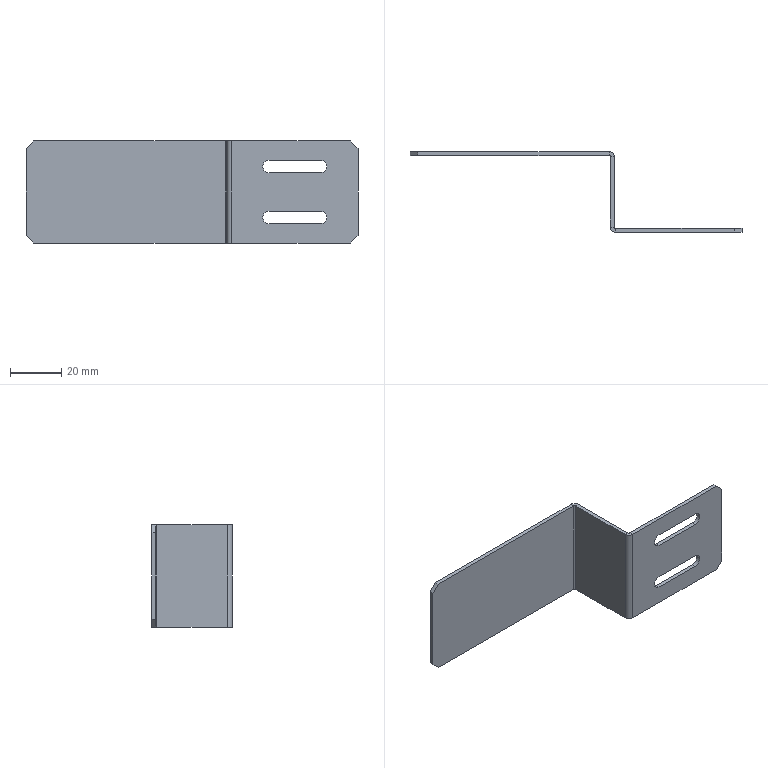Part | SolidWorks | features Chamfer 1, Cut 1, FlatPattern 1, SMBaseFlange 1, SheetMetal 1 | 1 solid | 34 faces | box 130 x 31.5 x 40 mm | volume 9150 mm3 | plane 26 | cylinder 8 | commonest cylinder face diameters 5 x4 1 x2 4 x2
STEP:
#1=CARTESIAN_POINT('',(0.,13.,20.));
#2=VERTEX_POINT('',#1);
#3=CARTESIAN_POINT('',(-1.5,13.,20.));
#4=VERTEX_POINT('',#3);
#5=CARTESIAN_POINT('',(0.,13.,20.));
#6=DIRECTION('',(-1.,0.,0.));
#7=VECTOR('',#6,1000.);
#8=LINE('',#5,#7);
#9=EDGE_CURVE('',#2,#4,#8,.T.);
#10=ORIENTED_EDGE('',*,*,#9,.F.);
#11=CARTESIAN_POINT('',(-2.,15.,20.));
#12=VERTEX_POINT('',#11);
#13=CARTESIAN_POINT('',(-2.,13.,20.));
#14=DIRECTION('',(0.,0.,-1.));
#15=DIRECTION('',(1.,0.,0.));
#16=AXIS2_PLACEMENT_3D('',#13,#14,#15);
#17=CIRCLE('',#16,2.);
#18=EDGE_CURVE('',#12,#2,#17,.T.);
#19=ORIENTED_EDGE('',*,*,#18,.F.);
#20=CARTESIAN_POINT('',(-2.,13.5,20.));
#21=VERTEX_POINT('',#20);
#22=CARTESIAN_POINT('',(-2.,13.5,20.));
#23=DIRECTION('',(0.,1.,0.));
#24=VECTOR('',#23,1000.);
#25=LINE('',#22,#24);
#26=EDGE_CURVE('',#21,#12,#25,.T.);
#27=ORIENTED_EDGE('',*,*,#26,.F.);
#28=CARTESIAN_POINT('',(-2.,13.,20.));
#29=DIRECTION('',(0.,0.,-1.));
#30=DIRECTION('',(1.,0.,0.));
#31=AXIS2_PLACEMENT_3D('',#28,#29,#30);
#32=CIRCLE('',#31,0.5);
#33=EDGE_CURVE('',#21,#4,#32,.T.);
#34=ORIENTED_EDGE('',*,*,#33,.T.);
#35=EDGE_LOOP('',(#10,#19,#27,#34));
#36=FACE_OUTER_BOUND('',#35,.T.);
#37=CARTESIAN_POINT('',(0.,13.,20.));
#38=DIRECTION('',(0.,0.,1.));
#39=DIRECTION('',(1.,0.,0.));
#40=AXIS2_PLACEMENT_3D('',#37,#38,#39);
#41=PLANE('',#40);
#42=ADVANCED_FACE('',(#36),#41,.T.);
#43=CARTESIAN_POINT('',(0.,-14.5,20.));
#44=VERTEX_POINT('',#43);
#45=CARTESIAN_POINT('',(0.,15.,20.));
#46=DIRECTION('',(0.,-1.,0.));
#47=VECTOR('',#46,1000.);
#48=LINE('',#45,#47);
#49=EDGE_CURVE('',#2,#44,#48,.T.);
#50=ORIENTED_EDGE('',*,*,#49,.F.);
#51=ORIENTED_EDGE('',*,*,#9,.T.);
#52=CARTESIAN_POINT('',(-1.5,-14.5,20.));
#53=VERTEX_POINT('',#52);
#54=CARTESIAN_POINT('',(-1.5,15.,20.));
#55=DIRECTION('',(0.,-1.,0.));
#56=VECTOR('',#55,1000.);
#57=LINE('',#54,#56);
#58=EDGE_CURVE('',#4,#53,#57,.T.);
#59=ORIENTED_EDGE('',*,*,#58,.T.);
#60=CARTESIAN_POINT('',(-1.5,-14.5,20.));
#61=DIRECTION('',(1.,0.,0.));
#62=VECTOR('',#61,1000.);
#63=LINE('',#60,#62);
#64=EDGE_CURVE('',#53,#44,#63,.T.);
#65=ORIENTED_EDGE('',*,*,#64,.T.);
#66=EDGE_LOOP('',(#50,#51,#59,#65));
#67=FACE_OUTER_BOUND('',#66,.T.);
#68=CARTESIAN_POINT('',(-2.,13.5,20.));
#69=DIRECTION('',(0.,0.,1.));
#70=DIRECTION('',(1.,0.,0.));
#71=AXIS2_PLACEMENT_3D('',#68,#69,#70);
#72=PLANE('',#71);
#73=ADVANCED_FACE('',(#67),#72,.T.);
#74=CARTESIAN_POINT('',(-2.,15.,-20.));
#75=VERTEX_POINT('',#74);
#76=CARTESIAN_POINT('',(-2.,13.5,-20.));
#77=VERTEX_POINT('',#76);
#78=CARTESIAN_POINT('',(-2.,15.,-20.));
#79=DIRECTION('',(0.,-1.,0.));
#80=VECTOR('',#79,1000.);
#81=LINE('',#78,#80);
#82=EDGE_CURVE('',#75,#77,#81,.T.);
#83=ORIENTED_EDGE('',*,*,#82,.F.);
#84=CARTESIAN_POINT('',(0.,13.,-20.));
#85=VERTEX_POINT('',#84);
#86=CARTESIAN_POINT('',(-2.,13.,-20.));
#87=DIRECTION('',(0.,0.,-1.));
#88=DIRECTION('',(1.,0.,0.));
#89=AXIS2_PLACEMENT_3D('',#86,#87,#88);
#90=CIRCLE('',#89,2.);
#91=EDGE_CURVE('',#75,#85,#90,.T.);
#92=ORIENTED_EDGE('',*,*,#91,.T.);
#93=CARTESIAN_POINT('',(-1.5,13.,-20.));
#94=VERTEX_POINT('',#93);
#95=CARTESIAN_POINT('',(-1.5,13.,-20.));
#96=DIRECTION('',(1.,0.,0.));
#97=VECTOR('',#96,1000.);
#98=LINE('',#95,#97);
#99=EDGE_CURVE('',#94,#85,#98,.T.);
#100=ORIENTED_EDGE('',*,*,#99,.F.);
#101=CARTESIAN_POINT('',(-2.,13.,-20.));
#102=DIRECTION('',(0.,0.,-1.));
#103=DIRECTION('',(1.,0.,0.));
#104=AXIS2_PLACEMENT_3D('',#101,#102,#103);
#105=CIRCLE('',#104,0.5);
#106=EDGE_CURVE('',#77,#94,#105,.T.);
#107=ORIENTED_EDGE('',*,*,#106,.F.);
#108=EDGE_LOOP('',(#83,#92,#100,#107));
#109=FACE_OUTER_BOUND('',#108,.T.);
#110=CARTESIAN_POINT('',(-2.,15.,-20.));
#111=DIRECTION('',(0.,0.,-1.));
#112=DIRECTION('',(-1.,0.,0.));
#113=AXIS2_PLACEMENT_3D('',#110,#111,#112);
#114=PLANE('',#113);
#115=ADVANCED_FACE('',(#109),#114,.T.);
#116=CARTESIAN_POINT('',(-77.,13.5,-20.));
#117=VERTEX_POINT('',#116);
#118=CARTESIAN_POINT('',(-80.,13.5,-20.));
#119=DIRECTION('',(1.,0.,0.));
#120=VECTOR('',#119,1000.);
#121=LINE('',#118,#120);
#122=EDGE_CURVE('',#117,#77,#121,.T.);
#123=ORIENTED_EDGE('',*,*,#122,.F.);
#124=CARTESIAN_POINT('',(-77.,15.,-20.));
#125=VERTEX_POINT('',#124);
#126=CARTESIAN_POINT('',(-77.,13.,-20.));
#127=DIRECTION('',(0.,1.,0.));
#128=VECTOR('',#127,1000.);
#129=LINE('',#126,#128);
#130=EDGE_CURVE('',#117,#125,#129,.T.);
#131=ORIENTED_EDGE('',*,*,#130,.T.);
#132=CARTESIAN_POINT('',(-80.,15.,-20.));
#133=DIRECTION('',(1.,0.,0.));
#134=VECTOR('',#133,1000.);
#135=LINE('',#132,#134);
#136=EDGE_CURVE('',#125,#75,#135,.T.);
#137=ORIENTED_EDGE('',*,*,#136,.T.);
#138=ORIENTED_EDGE('',*,*,#82,.T.);
#139=EDGE_LOOP('',(#123,#131,#137,#138));
#140=FACE_OUTER_BOUND('',#139,.T.);
#141=CARTESIAN_POINT('',(-1.5,13.,-20.));
#142=DIRECTION('',(0.,0.,-1.));
#143=DIRECTION('',(-1.,0.,0.));
#144=AXIS2_PLACEMENT_3D('',#141,#142,#143);
#145=PLANE('',#144);
#146=ADVANCED_FACE('',(#140),#145,.T.);
#147=CARTESIAN_POINT('',(0.5,-15.,20.));
#148=VERTEX_POINT('',#147);
#149=CARTESIAN_POINT('',(0.5,-16.5,20.));
#150=VERTEX_POINT('',#149);
#151=CARTESIAN_POINT('',(0.5,-15.,20.));
#152=DIRECTION('',(0.,-1.,0.));
#153=VECTOR('',#152,1000.);
#154=LINE('',#151,#153);
#155=EDGE_CURVE('',#148,#150,#154,.T.);
#156=ORIENTED_EDGE('',*,*,#155,.F.);
#157=CARTESIAN_POINT('',(0.5,-14.5,20.));
#158=DIRECTION('',(0.,0.,1.));
#159=DIRECTION('',(-1.,0.,0.));
#160=AXIS2_PLACEMENT_3D('',#157,#158,#159);
#161=CIRCLE('',#160,0.5);
#162=EDGE_CURVE('',#44,#148,#161,.T.);
#163=ORIENTED_EDGE('',*,*,#162,.F.);
#164=ORIENTED_EDGE('',*,*,#64,.F.);
#165=CARTESIAN_POINT('',(0.5,-14.5,20.));
#166=DIRECTION('',(0.,0.,1.));
#167=DIRECTION('',(1.,0.,0.));
#168=AXIS2_PLACEMENT_3D('',#165,#166,#167);
#169=CIRCLE('',#168,2.);
#170=EDGE_CURVE('',#53,#150,#169,.T.);
#171=ORIENTED_EDGE('',*,*,#170,.T.);
#172=EDGE_LOOP('',(#156,#163,#164,#171));
#173=FACE_OUTER_BOUND('',#172,.T.);
#174=CARTESIAN_POINT('',(0.5,-15.,20.));
#175=DIRECTION('',(0.,0.,1.));
#176=DIRECTION('',(1.,0.,0.));
#177=AXIS2_PLACEMENT_3D('',#174,#175,#176);
#178=PLANE('',#177);
#179=ADVANCED_FACE('',(#173),#178,.T.);
#180=CARTESIAN_POINT('',(47.,-16.5,20.));
#181=VERTEX_POINT('',#180);
#182=CARTESIAN_POINT('',(0.,-16.5,20.));
#183=DIRECTION('',(1.,0.,0.));
#184=VECTOR('',#183,1000.);
#185=LINE('',#182,#184);
#186=EDGE_CURVE('',#150,#181,#185,.T.);
#187=ORIENTED_EDGE('',*,*,#186,.T.);
#188=CARTESIAN_POINT('',(47.,-15.,20.));
#189=VERTEX_POINT('',#188);
#190=CARTESIAN_POINT('',(47.,-14.5,20.));
#191=DIRECTION('',(0.,1.,0.));
#192=VECTOR('',#191,1000.);
#193=LINE('',#190,#192);
#194=EDGE_CURVE('',#181,#189,#193,.T.);
#195=ORIENTED_EDGE('',*,*,#194,.T.);
#196=CARTESIAN_POINT('',(0.,-15.,20.));
#197=DIRECTION('',(1.,0.,0.));
#198=VECTOR('',#197,1000.);
#199=LINE('',#196,#198);
#200=EDGE_CURVE('',#148,#189,#199,.T.);
#201=ORIENTED_EDGE('',*,*,#200,.F.);
#202=ORIENTED_EDGE('',*,*,#155,.T.);
#203=EDGE_LOOP('',(#187,#195,#201,#202));
#204=FACE_OUTER_BOUND('',#203,.T.);
#205=CARTESIAN_POINT('',(-1.5,-14.5,20.));
#206=DIRECTION('',(0.,0.,1.));
#207=DIRECTION('',(1.,0.,0.));
#208=AXIS2_PLACEMENT_3D('',#205,#206,#207);
#209=PLANE('',#208);
#210=ADVANCED_FACE('',(#204),#209,.T.);
#211=CARTESIAN_POINT('',(0.,-14.5,-20.));
#212=VERTEX_POINT('',#211);
#213=CARTESIAN_POINT('',(-1.5,-14.5,-20.));
#214=VERTEX_POINT('',#213);
#215=CARTESIAN_POINT('',(0.,-14.5,-20.));
#216=DIRECTION('',(-1.,0.,0.));
#217=VECTOR('',#216,1000.);
#218=LINE('',#215,#217);
#219=EDGE_CURVE('',#212,#214,#218,.T.);
#220=ORIENTED_EDGE('',*,*,#219,.F.);
#221=CARTESIAN_POINT('',(0.5,-15.,-20.));
#222=VERTEX_POINT('',#221);
#223=CARTESIAN_POINT('',(0.5,-14.5,-20.));
#224=DIRECTION('',(0.,0.,1.));
#225=DIRECTION('',(-1.,0.,0.));
#226=AXIS2_PLACEMENT_3D('',#223,#224,#225);
#227=CIRCLE('',#226,0.5);
#228=EDGE_CURVE('',#212,#222,#227,.T.);
#229=ORIENTED_EDGE('',*,*,#228,.T.);
#230=CARTESIAN_POINT('',(0.5,-16.5,-20.));
#231=VERTEX_POINT('',#230);
#232=CARTESIAN_POINT('',(0.5,-16.5,-20.));
#233=DIRECTION('',(0.,1.,0.));
#234=VECTOR('',#233,1000.);
#235=LINE('',#232,#234);
#236=EDGE_CURVE('',#231,#222,#235,.T.);
#237=ORIENTED_EDGE('',*,*,#236,.F.);
#238=CARTESIAN_POINT('',(0.5,-14.5,-20.));
#239=DIRECTION('',(0.,0.,1.));
#240=DIRECTION('',(1.,0.,0.));
#241=AXIS2_PLACEMENT_3D('',#238,#239,#240);
#242=CIRCLE('',#241,2.);
#243=EDGE_CURVE('',#214,#231,#242,.T.);
#244=ORIENTED_EDGE('',*,*,#243,.F.);
#245=EDGE_LOOP('',(#220,#229,#237,#244));
#246=FACE_OUTER_BOUND('',#245,.T.);
#247=CARTESIAN_POINT('',(0.,-14.5,-20.));
#248=DIRECTION('',(0.,0.,-1.));
#249=DIRECTION('',(-1.,0.,0.));
#250=AXIS2_PLACEMENT_3D('',#247,#248,#249);
#251=PLANE('',#250);
#252=ADVANCED_FACE('',(#246),#251,.T.);
#253=CARTESIAN_POINT('',(0.,15.,-20.));
#254=DIRECTION('',(0.,-1.,0.));
#255=VECTOR('',#254,1000.);
#256=LINE('',#253,#255);
#257=EDGE_CURVE('',#85,#212,#256,.T.);
#258=ORIENTED_EDGE('',*,*,#257,.T.);
#259=ORIENTED_EDGE('',*,*,#219,.T.);
#260=CARTESIAN_POINT('',(-1.5,15.,-20.));
#261=DIRECTION('',(0.,-1.,0.));
#262=VECTOR('',#261,1000.);
#263=LINE('',#260,#262);
#264=EDGE_CURVE('',#94,#214,#263,.T.);
#265=ORIENTED_EDGE('',*,*,#264,.F.);
#266=ORIENTED_EDGE('',*,*,#99,.T.);
#267=EDGE_LOOP('',(#258,#259,#265,#266));
#268=FACE_OUTER_BOUND('',#267,.T.);
#269=CARTESIAN_POINT('',(0.5,-16.5,-20.));
#270=DIRECTION('',(0.,0.,-1.));
#271=DIRECTION('',(-1.,0.,0.));
#272=AXIS2_PLACEMENT_3D('',#269,#270,#271);
#273=PLANE('',#272);
#274=ADVANCED_FACE('',(#268),#273,.T.);
#275=CARTESIAN_POINT('',(15.25,-16.5,12.5));
#276=VERTEX_POINT('',#275);
#277=CARTESIAN_POINT('',(35.25,-16.5,12.5));
#278=VERTEX_POINT('',#277);
#279=CARTESIAN_POINT('',(35.25,-16.5,12.5));
#280=DIRECTION('',(1.,0.,0.));
#281=VECTOR('',#280,1000.);
#282=LINE('',#279,#281);
#283=EDGE_CURVE('',#276,#278,#282,.T.);
#284=ORIENTED_EDGE('',*,*,#283,.T.);
#285=CARTESIAN_POINT('',(35.25,-16.5,7.5));
#286=VERTEX_POINT('',#285);
#287=CARTESIAN_POINT('',(35.25,-16.5,10.));
#288=DIRECTION('',(0.,1.,0.));
#289=DIRECTION('',(0.,0.,1.));
#290=AXIS2_PLACEMENT_3D('',#287,#288,#289);
#291=CIRCLE('',#290,2.5);
#292=EDGE_CURVE('',#278,#286,#291,.T.);
#293=ORIENTED_EDGE('',*,*,#292,.T.);
#294=CARTESIAN_POINT('',(15.25,-16.5,7.5));
#295=VERTEX_POINT('',#294);
#296=CARTESIAN_POINT('',(35.25,-16.5,7.5));
#297=DIRECTION('',(-1.,0.,0.));
#298=VECTOR('',#297,1000.);
#299=LINE('',#296,#298);
#300=EDGE_CURVE('',#286,#295,#299,.T.);
#301=ORIENTED_EDGE('',*,*,#300,.T.);
#302=CARTESIAN_POINT('',(15.25,-16.5,10.));
#303=DIRECTION('',(0.,1.,0.));
#304=DIRECTION('',(0.,0.,1.));
#305=AXIS2_PLACEMENT_3D('',#302,#303,#304);
#306=CIRCLE('',#305,2.5);
#307=EDGE_CURVE('',#295,#276,#306,.T.);
#308=ORIENTED_EDGE('',*,*,#307,.T.);
#309=EDGE_LOOP('',(#284,#293,#301,#308));
#310=FACE_BOUND('',#309,.T.);
#311=CARTESIAN_POINT('',(15.25,-16.5,-7.5));
#312=VERTEX_POINT('',#311);
#313=CARTESIAN_POINT('',(35.25,-16.5,-7.5));
#314=VERTEX_POINT('',#313);
#315=CARTESIAN_POINT('',(35.25,-16.5,-7.5));
#316=DIRECTION('',(1.,0.,0.));
#317=VECTOR('',#316,1000.);
#318=LINE('',#315,#317);
#319=EDGE_CURVE('',#312,#314,#318,.T.);
#320=ORIENTED_EDGE('',*,*,#319,.T.);
#321=CARTESIAN_POINT('',(35.25,-16.5,-12.5));
#322=VERTEX_POINT('',#321);
#323=CARTESIAN_POINT('',(35.25,-16.5,-10.));
#324=DIRECTION('',(0.,1.,0.));
#325=DIRECTION('',(0.,0.,1.));
#326=AXIS2_PLACEMENT_3D('',#323,#324,#325);
#327=CIRCLE('',#326,2.5);
#328=EDGE_CURVE('',#314,#322,#327,.T.);
#329=ORIENTED_EDGE('',*,*,#328,.T.);
#330=CARTESIAN_POINT('',(15.25,-16.5,-12.5));
#331=VERTEX_POINT('',#330);
#332=CARTESIAN_POINT('',(35.25,-16.5,-12.5));
#333=DIRECTION('',(-1.,0.,0.));
#334=VECTOR('',#333,1000.);
#335=LINE('',#332,#334);
#336=EDGE_CURVE('',#322,#331,#335,.T.);
#337=ORIENTED_EDGE('',*,*,#336,.T.);
#338=CARTESIAN_POINT('',(15.25,-16.5,-10.));
#339=DIRECTION('',(0.,1.,0.));
#340=DIRECTION('',(0.,0.,1.));
#341=AXIS2_PLACEMENT_3D('',#338,#339,#340);
#342=CIRCLE('',#341,2.5);
#343=EDGE_CURVE('',#331,#312,#342,.T.);
#344=ORIENTED_EDGE('',*,*,#343,.T.);
#345=EDGE_LOOP('',(#320,#329,#337,#344));
#346=FACE_BOUND('',#345,.T.);
#347=CARTESIAN_POINT('',(47.,-16.5,-20.));
#348=VERTEX_POINT('',#347);
#349=CARTESIAN_POINT('',(0.,-16.5,-20.));
#350=DIRECTION('',(1.,0.,0.));
#351=VECTOR('',#350,1000.);
#352=LINE('',#349,#351);
#353=EDGE_CURVE('',#231,#348,#352,.T.);
#354=ORIENTED_EDGE('',*,*,#353,.T.);
#355=CARTESIAN_POINT('',(50.,-16.5,-17.));
#356=VERTEX_POINT('',#355);
#357=CARTESIAN_POINT('',(47.,-16.5,-20.));
#358=DIRECTION('',(0.7071,0.,0.7071));
#359=VECTOR('',#358,1000.);
#360=LINE('',#357,#359);
#361=EDGE_CURVE('',#348,#356,#360,.T.);
#362=ORIENTED_EDGE('',*,*,#361,.T.);
#363=CARTESIAN_POINT('',(50.,-16.5,17.));
#364=VERTEX_POINT('',#363);
#365=CARTESIAN_POINT('',(50.,-16.5,20.));
#366=DIRECTION('',(0.,0.,-1.));
#367=VECTOR('',#366,1000.);
#368=LINE('',#365,#367);
#369=EDGE_CURVE('',#364,#356,#368,.T.);
#370=ORIENTED_EDGE('',*,*,#369,.F.);
#371=CARTESIAN_POINT('',(50.,-16.5,17.));
#372=DIRECTION('',(-0.7071,0.,0.7071));
#373=VECTOR('',#372,1000.);
#374=LINE('',#371,#373);
#375=EDGE_CURVE('',#364,#181,#374,.T.);
#376=ORIENTED_EDGE('',*,*,#375,.T.);
#377=ORIENTED_EDGE('',*,*,#186,.F.);
#378=CARTESIAN_POINT('',(0.5,-16.5,20.));
#379=DIRECTION('',(0.,0.,-1.));
#380=VECTOR('',#379,1000.);
#381=LINE('',#378,#380);
#382=EDGE_CURVE('',#150,#231,#381,.T.);
#383=ORIENTED_EDGE('',*,*,#382,.T.);
#384=EDGE_LOOP('',(#354,#362,#370,#376,#377,#383));
#385=FACE_OUTER_BOUND('',#384,.T.);
#386=CARTESIAN_POINT('',(0.,-16.5,20.));
#387=DIRECTION('',(0.,1.,0.));
#388=DIRECTION('',(0.,0.,1.));
#389=AXIS2_PLACEMENT_3D('',#386,#387,#388);
#390=PLANE('',#389);
#391=ADVANCED_FACE('',(#310,#346,#385),#390,.F.);
#392=ORIENTED_EDGE('',*,*,#369,.T.);
#393=CARTESIAN_POINT('',(50.,-15.,-17.));
#394=VERTEX_POINT('',#393);
#395=CARTESIAN_POINT('',(50.,-15.,-17.));
#396=DIRECTION('',(0.,1.,0.));
#397=VECTOR('',#396,1000.);
#398=LINE('',#395,#397);
#399=EDGE_CURVE('',#356,#394,#398,.T.);
#400=ORIENTED_EDGE('',*,*,#399,.T.);
#401=CARTESIAN_POINT('',(50.,-15.,17.));
#402=VERTEX_POINT('',#401);
#403=CARTESIAN_POINT('',(50.,-15.,20.));
#404=DIRECTION('',(0.,0.,-1.));
#405=VECTOR('',#404,1000.);
#406=LINE('',#403,#405);
#407=EDGE_CURVE('',#402,#394,#406,.T.);
#408=ORIENTED_EDGE('',*,*,#407,.F.);
#409=CARTESIAN_POINT('',(50.,-15.,17.));
#410=DIRECTION('',(0.,-1.,0.));
#411=VECTOR('',#410,1000.);
#412=LINE('',#409,#411);
#413=EDGE_CURVE('',#402,#364,#412,.T.);
#414=ORIENTED_EDGE('',*,*,#413,.T.);
#415=EDGE_LOOP('',(#392,#400,#408,#414));
#416=FACE_OUTER_BOUND('',#415,.T.);
#417=CARTESIAN_POINT('',(50.,-15.,20.));
#418=DIRECTION('',(1.,0.,0.));
#419=DIRECTION('',(0.,0.,-1.));
#420=AXIS2_PLACEMENT_3D('',#417,#418,#419);
#421=PLANE('',#420);
#422=ADVANCED_FACE('',(#416),#421,.T.);
#423=CARTESIAN_POINT('',(35.25,-15.,12.5));
#424=VERTEX_POINT('',#423);
#425=CARTESIAN_POINT('',(35.25,-15.,7.5));
#426=VERTEX_POINT('',#425);
#427=CARTESIAN_POINT('',(35.25,-15.,10.));
#428=DIRECTION('',(0.,1.,0.));
#429=DIRECTION('',(0.,0.,1.));
#430=AXIS2_PLACEMENT_3D('',#427,#428,#429);
#431=CIRCLE('',#430,2.5);
#432=EDGE_CURVE('',#424,#426,#431,.T.);
#433=ORIENTED_EDGE('',*,*,#432,.F.);
#434=CARTESIAN_POINT('',(15.25,-15.,12.5));
#435=VERTEX_POINT('',#434);
#436=CARTESIAN_POINT('',(35.25,-15.,12.5));
#437=DIRECTION('',(1.,0.,0.));
#438=VECTOR('',#437,1000.);
#439=LINE('',#436,#438);
#440=EDGE_CURVE('',#435,#424,#439,.T.);
#441=ORIENTED_EDGE('',*,*,#440,.F.);
#442=CARTESIAN_POINT('',(15.25,-15.,7.5));
#443=VERTEX_POINT('',#442);
#444=CARTESIAN_POINT('',(15.25,-15.,10.));
#445=DIRECTION('',(0.,1.,0.));
#446=DIRECTION('',(0.,0.,1.));
#447=AXIS2_PLACEMENT_3D('',#444,#445,#446);
#448=CIRCLE('',#447,2.5);
#449=EDGE_CURVE('',#443,#435,#448,.T.);
#450=ORIENTED_EDGE('',*,*,#449,.F.);
#451=CARTESIAN_POINT('',(35.25,-15.,7.5));
#452=DIRECTION('',(-1.,0.,0.));
#453=VECTOR('',#452,1000.);
#454=LINE('',#451,#453);
#455=EDGE_CURVE('',#426,#443,#454,.T.);
#456=ORIENTED_EDGE('',*,*,#455,.F.);
#457=EDGE_LOOP('',(#433,#441,#450,#456));
#458=FACE_BOUND('',#457,.T.);
#459=CARTESIAN_POINT('',(35.25,-15.,-7.5));
#460=VERTEX_POINT('',#459);
#461=CARTESIAN_POINT('',(35.25,-15.,-12.5));
#462=VERTEX_POINT('',#461);
#463=CARTESIAN_POINT('',(35.25,-15.,-10.));
#464=DIRECTION('',(0.,1.,0.));
#465=DIRECTION('',(0.,0.,1.));
#466=AXIS2_PLACEMENT_3D('',#463,#464,#465);
#467=CIRCLE('',#466,2.5);
#468=EDGE_CURVE('',#460,#462,#467,.T.);
#469=ORIENTED_EDGE('',*,*,#468,.F.);
#470=CARTESIAN_POINT('',(15.25,-15.,-7.5));
#471=VERTEX_POINT('',#470);
#472=CARTESIAN_POINT('',(35.25,-15.,-7.5));
#473=DIRECTION('',(1.,0.,0.));
#474=VECTOR('',#473,1000.);
#475=LINE('',#472,#474);
#476=EDGE_CURVE('',#471,#460,#475,.T.);
#477=ORIENTED_EDGE('',*,*,#476,.F.);
#478=CARTESIAN_POINT('',(15.25,-15.,-12.5));
#479=VERTEX_POINT('',#478);
#480=CARTESIAN_POINT('',(15.25,-15.,-10.));
#481=DIRECTION('',(0.,1.,0.));
#482=DIRECTION('',(0.,0.,1.));
#483=AXIS2_PLACEMENT_3D('',#480,#481,#482);
#484=CIRCLE('',#483,2.5);
#485=EDGE_CURVE('',#479,#471,#484,.T.);
#486=ORIENTED_EDGE('',*,*,#485,.F.);
#487=CARTESIAN_POINT('',(35.25,-15.,-12.5));
#488=DIRECTION('',(-1.,0.,0.));
#489=VECTOR('',#488,1000.);
#490=LINE('',#487,#489);
#491=EDGE_CURVE('',#462,#479,#490,.T.);
#492=ORIENTED_EDGE('',*,*,#491,.F.);
#493=EDGE_LOOP('',(#469,#477,#486,#492));
#494=FACE_BOUND('',#493,.T.);
#495=ORIENTED_EDGE('',*,*,#407,.T.);
#496=CARTESIAN_POINT('',(47.,-15.,-20.));
#497=VERTEX_POINT('',#496);
#498=CARTESIAN_POINT('',(43.5,-15.,-23.5));
#499=DIRECTION('',(-0.7071,0.,-0.7071));
#500=VECTOR('',#499,1000.);
#501=LINE('',#498,#500);
#502=EDGE_CURVE('',#394,#497,#501,.T.);
#503=ORIENTED_EDGE('',*,*,#502,.T.);
#504=CARTESIAN_POINT('',(0.,-15.,-20.));
#505=DIRECTION('',(1.,0.,0.));
#506=VECTOR('',#505,1000.);
#507=LINE('',#504,#506);
#508=EDGE_CURVE('',#222,#497,#507,.T.);
#509=ORIENTED_EDGE('',*,*,#508,.F.);
#510=CARTESIAN_POINT('',(0.5,-15.,20.));
#511=DIRECTION('',(0.,0.,-1.));
#512=VECTOR('',#511,1000.);
#513=LINE('',#510,#512);
#514=EDGE_CURVE('',#148,#222,#513,.T.);
#515=ORIENTED_EDGE('',*,*,#514,.F.);
#516=ORIENTED_EDGE('',*,*,#200,.T.);
#517=CARTESIAN_POINT('',(23.5,-15.,43.5));
#518=DIRECTION('',(0.7071,0.,-0.7071));
#519=VECTOR('',#518,1000.);
#520=LINE('',#517,#519);
#521=EDGE_CURVE('',#189,#402,#520,.T.);
#522=ORIENTED_EDGE('',*,*,#521,.T.);
#523=EDGE_LOOP('',(#495,#503,#509,#515,#516,#522));
#524=FACE_OUTER_BOUND('',#523,.T.);
#525=CARTESIAN_POINT('',(0.,-15.,20.));
#526=DIRECTION('',(0.,1.,0.));
#527=DIRECTION('',(0.,0.,1.));
#528=AXIS2_PLACEMENT_3D('',#525,#526,#527);
#529=PLANE('',#528);
#530=ADVANCED_FACE('',(#458,#494,#524),#529,.T.);
#531=ORIENTED_EDGE('',*,*,#228,.F.);
#532=CARTESIAN_POINT('',(0.,-14.5,20.));
#533=DIRECTION('',(0.,0.,-1.));
#534=VECTOR('',#533,1000.);
#535=LINE('',#532,#534);
#536=EDGE_CURVE('',#44,#212,#535,.T.);
#537=ORIENTED_EDGE('',*,*,#536,.F.);
#538=ORIENTED_EDGE('',*,*,#162,.T.);
#539=ORIENTED_EDGE('',*,*,#514,.T.);
#540=EDGE_LOOP('',(#531,#537,#538,#539));
#541=FACE_OUTER_BOUND('',#540,.T.);
#542=CARTESIAN_POINT('',(0.5,-14.5,20.));
#543=DIRECTION('',(0.,0.,-1.));
#544=DIRECTION('',(-1.,0.,0.));
#545=AXIS2_PLACEMENT_3D('',#542,#543,#544);
#546=CYLINDRICAL_SURFACE('',#545,0.5);
#547=ADVANCED_FACE('',(#541),#546,.F.);
#548=ORIENTED_EDGE('',*,*,#257,.F.);
#549=CARTESIAN_POINT('',(0.,13.,20.));
#550=DIRECTION('',(0.,0.,-1.));
#551=VECTOR('',#550,1000.);
#552=LINE('',#549,#551);
#553=EDGE_CURVE('',#2,#85,#552,.T.);
#554=ORIENTED_EDGE('',*,*,#553,.F.);
#555=ORIENTED_EDGE('',*,*,#49,.T.);
#556=ORIENTED_EDGE('',*,*,#536,.T.);
#557=EDGE_LOOP('',(#548,#554,#555,#556));
#558=FACE_OUTER_BOUND('',#557,.T.);
#559=CARTESIAN_POINT('',(0.,15.,20.));
#560=DIRECTION('',(1.,0.,0.));
#561=DIRECTION('',(0.,0.,-1.));
#562=AXIS2_PLACEMENT_3D('',#559,#560,#561);
#563=PLANE('',#562);
#564=ADVANCED_FACE('',(#558),#563,.T.);
#565=ORIENTED_EDGE('',*,*,#91,.F.);
#566=CARTESIAN_POINT('',(-2.,15.,20.));
#567=DIRECTION('',(0.,0.,-1.));
#568=VECTOR('',#567,1000.);
#569=LINE('',#566,#568);
#570=EDGE_CURVE('',#12,#75,#569,.T.);
#571=ORIENTED_EDGE('',*,*,#570,.F.);
#572=ORIENTED_EDGE('',*,*,#18,.T.);
#573=ORIENTED_EDGE('',*,*,#553,.T.);
#574=EDGE_LOOP('',(#565,#571,#572,#573));
#575=FACE_OUTER_BOUND('',#574,.T.);
#576=CARTESIAN_POINT('',(-2.,13.,20.));
#577=DIRECTION('',(0.,0.,-1.));
#578=DIRECTION('',(-1.,0.,0.));
#579=AXIS2_PLACEMENT_3D('',#576,#577,#578);
#580=CYLINDRICAL_SURFACE('',#579,2.);
#581=ADVANCED_FACE('',(#575),#580,.T.);
#582=ORIENTED_EDGE('',*,*,#136,.F.);
#583=CARTESIAN_POINT('',(-80.,15.,-17.));
#584=VERTEX_POINT('',#583);
#585=CARTESIAN_POINT('',(-98.5,15.,1.5));
#586=DIRECTION('',(-0.7071,0.,0.7071));
#587=VECTOR('',#586,1000.);
#588=LINE('',#585,#587);
#589=EDGE_CURVE('',#125,#584,#588,.T.);
#590=ORIENTED_EDGE('',*,*,#589,.T.);
#591=CARTESIAN_POINT('',(-80.,15.,17.));
#592=VERTEX_POINT('',#591);
#593=CARTESIAN_POINT('',(-80.,15.,20.));
#594=DIRECTION('',(0.,0.,-1.));
#595=VECTOR('',#594,1000.);
#596=LINE('',#593,#595);
#597=EDGE_CURVE('',#592,#584,#596,.T.);
#598=ORIENTED_EDGE('',*,*,#597,.F.);
#599=CARTESIAN_POINT('',(-77.,15.,20.));
#600=VERTEX_POINT('',#599);
#601=CARTESIAN_POINT('',(-78.5,15.,18.5));
#602=DIRECTION('',(0.7071,0.,0.7071));
#603=VECTOR('',#602,1000.);
#604=LINE('',#601,#603);
#605=EDGE_CURVE('',#592,#600,#604,.T.);
#606=ORIENTED_EDGE('',*,*,#605,.T.);
#607=CARTESIAN_POINT('',(-80.,15.,20.));
#608=DIRECTION('',(1.,0.,0.));
#609=VECTOR('',#608,1000.);
#610=LINE('',#607,#609);
#611=EDGE_CURVE('',#600,#12,#610,.T.);
#612=ORIENTED_EDGE('',*,*,#611,.T.);
#613=ORIENTED_EDGE('',*,*,#570,.T.);
#614=EDGE_LOOP('',(#582,#590,#598,#606,#612,#613));
#615=FACE_OUTER_BOUND('',#614,.T.);
#616=CARTESIAN_POINT('',(-80.,15.,20.));
#617=DIRECTION('',(0.,1.,0.));
#618=DIRECTION('',(0.,0.,1.));
#619=AXIS2_PLACEMENT_3D('',#616,#617,#618);
#620=PLANE('',#619);
#621=ADVANCED_FACE('',(#615),#620,.T.);
#622=ORIENTED_EDGE('',*,*,#597,.T.);
#623=CARTESIAN_POINT('',(-80.,13.5,-17.));
#624=VERTEX_POINT('',#623);
#625=CARTESIAN_POINT('',(-80.,13.5,-17.));
#626=DIRECTION('',(0.,-1.,0.));
#627=VECTOR('',#626,1000.);
#628=LINE('',#625,#627);
#629=EDGE_CURVE('',#584,#624,#628,.T.);
#630=ORIENTED_EDGE('',*,*,#629,.T.);
#631=CARTESIAN_POINT('',(-80.,13.5,17.));
#632=VERTEX_POINT('',#631);
#633=CARTESIAN_POINT('',(-80.,13.5,20.));
#634=DIRECTION('',(0.,0.,-1.));
#635=VECTOR('',#634,1000.);
#636=LINE('',#633,#635);
#637=EDGE_CURVE('',#632,#624,#636,.T.);
#638=ORIENTED_EDGE('',*,*,#637,.F.);
#639=CARTESIAN_POINT('',(-80.,15.,17.));
#640=DIRECTION('',(0.,1.,0.));
#641=VECTOR('',#640,1000.);
#642=LINE('',#639,#641);
#643=EDGE_CURVE('',#632,#592,#642,.T.);
#644=ORIENTED_EDGE('',*,*,#643,.T.);
#645=EDGE_LOOP('',(#622,#630,#638,#644));
#646=FACE_OUTER_BOUND('',#645,.T.);
#647=CARTESIAN_POINT('',(-80.,13.5,20.));
#648=DIRECTION('',(-1.,0.,0.));
#649=DIRECTION('',(0.,0.,1.));
#650=AXIS2_PLACEMENT_3D('',#647,#648,#649);
#651=PLANE('',#650);
#652=ADVANCED_FACE('',(#646),#651,.T.);
#653=ORIENTED_EDGE('',*,*,#637,.T.);
#654=CARTESIAN_POINT('',(-77.,13.5,-20.));
#655=DIRECTION('',(0.7071,0.,-0.7071));
#656=VECTOR('',#655,1000.);
#657=LINE('',#654,#656);
#658=EDGE_CURVE('',#624,#117,#657,.T.);
#659=ORIENTED_EDGE('',*,*,#658,.T.);
#660=ORIENTED_EDGE('',*,*,#122,.T.);
#661=CARTESIAN_POINT('',(-2.,13.5,20.));
#662=DIRECTION('',(0.,0.,-1.));
#663=VECTOR('',#662,1000.);
#664=LINE('',#661,#663);
#665=EDGE_CURVE('',#21,#77,#664,.T.);
#666=ORIENTED_EDGE('',*,*,#665,.F.);
#667=CARTESIAN_POINT('',(-77.,13.5,20.));
#668=VERTEX_POINT('',#667);
#669=CARTESIAN_POINT('',(-80.,13.5,20.));
#670=DIRECTION('',(1.,0.,0.));
#671=VECTOR('',#670,1000.);
#672=LINE('',#669,#671);
#673=EDGE_CURVE('',#668,#21,#672,.T.);
#674=ORIENTED_EDGE('',*,*,#673,.F.);
#675=CARTESIAN_POINT('',(-80.,13.5,17.));
#676=DIRECTION('',(-0.7071,0.,-0.7071));
#677=VECTOR('',#676,1000.);
#678=LINE('',#675,#677);
#679=EDGE_CURVE('',#668,#632,#678,.T.);
#680=ORIENTED_EDGE('',*,*,#679,.T.);
#681=EDGE_LOOP('',(#653,#659,#660,#666,#674,#680));
#682=FACE_OUTER_BOUND('',#681,.T.);
#683=CARTESIAN_POINT('',(-80.,13.5,20.));
#684=DIRECTION('',(0.,1.,0.));
#685=DIRECTION('',(0.,0.,1.));
#686=AXIS2_PLACEMENT_3D('',#683,#684,#685);
#687=PLANE('',#686);
#688=ADVANCED_FACE('',(#682),#687,.F.);
#689=ORIENTED_EDGE('',*,*,#106,.T.);
#690=CARTESIAN_POINT('',(-1.5,13.,20.));
#691=DIRECTION('',(0.,0.,-1.));
#692=VECTOR('',#691,1000.);
#693=LINE('',#690,#692);
#694=EDGE_CURVE('',#4,#94,#693,.T.);
#695=ORIENTED_EDGE('',*,*,#694,.F.);
#696=ORIENTED_EDGE('',*,*,#33,.F.);
#697=ORIENTED_EDGE('',*,*,#665,.T.);
#698=EDGE_LOOP('',(#689,#695,#696,#697));
#699=FACE_OUTER_BOUND('',#698,.T.);
#700=CARTESIAN_POINT('',(-2.,13.,20.));
#701=DIRECTION('',(0.,0.,-1.));
#702=DIRECTION('',(-1.,0.,0.));
#703=AXIS2_PLACEMENT_3D('',#700,#701,#702);
#704=CYLINDRICAL_SURFACE('',#703,0.5);
#705=ADVANCED_FACE('',(#699),#704,.F.);
#706=ORIENTED_EDGE('',*,*,#264,.T.);
#707=CARTESIAN_POINT('',(-1.5,-14.5,20.));
#708=DIRECTION('',(0.,0.,-1.));
#709=VECTOR('',#708,1000.);
#710=LINE('',#707,#709);
#711=EDGE_CURVE('',#53,#214,#710,.T.);
#712=ORIENTED_EDGE('',*,*,#711,.F.);
#713=ORIENTED_EDGE('',*,*,#58,.F.);
#714=ORIENTED_EDGE('',*,*,#694,.T.);
#715=EDGE_LOOP('',(#706,#712,#713,#714));
#716=FACE_OUTER_BOUND('',#715,.T.);
#717=CARTESIAN_POINT('',(-1.5,15.,20.));
#718=DIRECTION('',(1.,0.,0.));
#719=DIRECTION('',(0.,0.,-1.));
#720=AXIS2_PLACEMENT_3D('',#717,#718,#719);
#721=PLANE('',#720);
#722=ADVANCED_FACE('',(#716),#721,.F.);
#723=ORIENTED_EDGE('',*,*,#243,.T.);
#724=ORIENTED_EDGE('',*,*,#382,.F.);
#725=ORIENTED_EDGE('',*,*,#170,.F.);
#726=ORIENTED_EDGE('',*,*,#711,.T.);
#727=EDGE_LOOP('',(#723,#724,#725,#726));
#728=FACE_OUTER_BOUND('',#727,.T.);
#729=CARTESIAN_POINT('',(0.5,-14.5,20.));
#730=DIRECTION('',(0.,0.,-1.));
#731=DIRECTION('',(-1.,0.,0.));
#732=AXIS2_PLACEMENT_3D('',#729,#730,#731);
#733=CYLINDRICAL_SURFACE('',#732,2.);
#734=ADVANCED_FACE('',(#728),#733,.T.);
#735=ORIENTED_EDGE('',*,*,#611,.F.);
#736=CARTESIAN_POINT('',(-77.,13.5,20.));
#737=DIRECTION('',(0.,-1.,0.));
#738=VECTOR('',#737,1000.);
#739=LINE('',#736,#738);
#740=EDGE_CURVE('',#600,#668,#739,.T.);
#741=ORIENTED_EDGE('',*,*,#740,.T.);
#742=ORIENTED_EDGE('',*,*,#673,.T.);
#743=ORIENTED_EDGE('',*,*,#26,.T.);
#744=EDGE_LOOP('',(#735,#741,#742,#743));
#745=FACE_OUTER_BOUND('',#744,.T.);
#746=CARTESIAN_POINT('',(0.5,-14.5,20.));
#747=DIRECTION('',(0.,0.,-1.));
#748=DIRECTION('',(-1.,0.,0.));
#749=AXIS2_PLACEMENT_3D('',#746,#747,#748);
#750=PLANE('',#749);
#751=ADVANCED_FACE('',(#745),#750,.F.);
#752=ORIENTED_EDGE('',*,*,#508,.T.);
#753=CARTESIAN_POINT('',(47.,-14.5,-20.));
#754=DIRECTION('',(0.,-1.,0.));
#755=VECTOR('',#754,1000.);
#756=LINE('',#753,#755);
#757=EDGE_CURVE('',#497,#348,#756,.T.);
#758=ORIENTED_EDGE('',*,*,#757,.T.);
#759=ORIENTED_EDGE('',*,*,#353,.F.);
#760=ORIENTED_EDGE('',*,*,#236,.T.);
#761=EDGE_LOOP('',(#752,#758,#759,#760));
#762=FACE_OUTER_BOUND('',#761,.T.);
#763=CARTESIAN_POINT('',(0.5,-14.5,-20.));
#764=DIRECTION('',(0.,0.,-1.));
#765=DIRECTION('',(-1.,0.,0.));
#766=AXIS2_PLACEMENT_3D('',#763,#764,#765);
#767=PLANE('',#766);
#768=ADVANCED_FACE('',(#762),#767,.T.);
#769=ORIENTED_EDGE('',*,*,#468,.T.);
#770=CARTESIAN_POINT('',(35.25,-16.5,-12.5));
#771=DIRECTION('',(0.,1.,0.));
#772=VECTOR('',#771,1000.);
#773=LINE('',#770,#772);
#774=EDGE_CURVE('',#322,#462,#773,.T.);
#775=ORIENTED_EDGE('',*,*,#774,.F.);
#776=ORIENTED_EDGE('',*,*,#328,.F.);
#777=CARTESIAN_POINT('',(35.25,-16.5,-7.5));
#778=DIRECTION('',(0.,1.,0.));
#779=VECTOR('',#778,1000.);
#780=LINE('',#777,#779);
#781=EDGE_CURVE('',#314,#460,#780,.T.);
#782=ORIENTED_EDGE('',*,*,#781,.T.);
#783=EDGE_LOOP('',(#769,#775,#776,#782));
#784=FACE_OUTER_BOUND('',#783,.T.);
#785=CARTESIAN_POINT('',(35.25,-16.5,-10.));
#786=DIRECTION('',(0.,1.,0.));
#787=DIRECTION('',(0.,0.,1.));
#788=AXIS2_PLACEMENT_3D('',#785,#786,#787);
#789=CYLINDRICAL_SURFACE('',#788,2.5);
#790=ADVANCED_FACE('',(#784),#789,.F.);
#791=ORIENTED_EDGE('',*,*,#476,.T.);
#792=ORIENTED_EDGE('',*,*,#781,.F.);
#793=ORIENTED_EDGE('',*,*,#319,.F.);
#794=CARTESIAN_POINT('',(15.25,-16.5,-7.5));
#795=DIRECTION('',(0.,1.,0.));
#796=VECTOR('',#795,1000.);
#797=LINE('',#794,#796);
#798=EDGE_CURVE('',#312,#471,#797,.T.);
#799=ORIENTED_EDGE('',*,*,#798,.T.);
#800=EDGE_LOOP('',(#791,#792,#793,#799));
#801=FACE_OUTER_BOUND('',#800,.T.);
#802=CARTESIAN_POINT('',(35.25,-16.5,-7.5));
#803=DIRECTION('',(0.,0.,1.));
#804=DIRECTION('',(1.,0.,0.));
#805=AXIS2_PLACEMENT_3D('',#802,#803,#804);
#806=PLANE('',#805);
#807=ADVANCED_FACE('',(#801),#806,.F.);
#808=ORIENTED_EDGE('',*,*,#485,.T.);
#809=ORIENTED_EDGE('',*,*,#798,.F.);
#810=ORIENTED_EDGE('',*,*,#343,.F.);
#811=CARTESIAN_POINT('',(15.25,-16.5,-12.5));
#812=DIRECTION('',(0.,1.,0.));
#813=VECTOR('',#812,1000.);
#814=LINE('',#811,#813);
#815=EDGE_CURVE('',#331,#479,#814,.T.);
#816=ORIENTED_EDGE('',*,*,#815,.T.);
#817=EDGE_LOOP('',(#808,#809,#810,#816));
#818=FACE_OUTER_BOUND('',#817,.T.);
#819=CARTESIAN_POINT('',(15.25,-16.5,-10.));
#820=DIRECTION('',(0.,1.,0.));
#821=DIRECTION('',(0.,0.,1.));
#822=AXIS2_PLACEMENT_3D('',#819,#820,#821);
#823=CYLINDRICAL_SURFACE('',#822,2.5);
#824=ADVANCED_FACE('',(#818),#823,.F.);
#825=ORIENTED_EDGE('',*,*,#491,.T.);
#826=ORIENTED_EDGE('',*,*,#815,.F.);
#827=ORIENTED_EDGE('',*,*,#336,.F.);
#828=ORIENTED_EDGE('',*,*,#774,.T.);
#829=EDGE_LOOP('',(#825,#826,#827,#828));
#830=FACE_OUTER_BOUND('',#829,.T.);
#831=CARTESIAN_POINT('',(35.25,-16.5,-12.5));
#832=DIRECTION('',(0.,0.,-1.));
#833=DIRECTION('',(-1.,0.,0.));
#834=AXIS2_PLACEMENT_3D('',#831,#832,#833);
#835=PLANE('',#834);
#836=ADVANCED_FACE('',(#830),#835,.F.);
#837=ORIENTED_EDGE('',*,*,#432,.T.);
#838=CARTESIAN_POINT('',(35.25,-16.5,7.5));
#839=DIRECTION('',(0.,1.,0.));
#840=VECTOR('',#839,1000.);
#841=LINE('',#838,#840);
#842=EDGE_CURVE('',#286,#426,#841,.T.);
#843=ORIENTED_EDGE('',*,*,#842,.F.);
#844=ORIENTED_EDGE('',*,*,#292,.F.);
#845=CARTESIAN_POINT('',(35.25,-16.5,12.5));
#846=DIRECTION('',(0.,1.,0.));
#847=VECTOR('',#846,1000.);
#848=LINE('',#845,#847);
#849=EDGE_CURVE('',#278,#424,#848,.T.);
#850=ORIENTED_EDGE('',*,*,#849,.T.);
#851=EDGE_LOOP('',(#837,#843,#844,#850));
#852=FACE_OUTER_BOUND('',#851,.T.);
#853=CARTESIAN_POINT('',(35.25,-16.5,10.));
#854=DIRECTION('',(0.,1.,0.));
#855=DIRECTION('',(0.,0.,1.));
#856=AXIS2_PLACEMENT_3D('',#853,#854,#855);
#857=CYLINDRICAL_SURFACE('',#856,2.5);
#858=ADVANCED_FACE('',(#852),#857,.F.);
#859=ORIENTED_EDGE('',*,*,#440,.T.);
#860=ORIENTED_EDGE('',*,*,#849,.F.);
#861=ORIENTED_EDGE('',*,*,#283,.F.);
#862=CARTESIAN_POINT('',(15.25,-16.5,12.5));
#863=DIRECTION('',(0.,1.,0.));
#864=VECTOR('',#863,1000.);
#865=LINE('',#862,#864);
#866=EDGE_CURVE('',#276,#435,#865,.T.);
#867=ORIENTED_EDGE('',*,*,#866,.T.);
#868=EDGE_LOOP('',(#859,#860,#861,#867));
#869=FACE_OUTER_BOUND('',#868,.T.);
#870=CARTESIAN_POINT('',(35.25,-16.5,12.5));
#871=DIRECTION('',(0.,0.,1.));
#872=DIRECTION('',(1.,0.,0.));
#873=AXIS2_PLACEMENT_3D('',#870,#871,#872);
#874=PLANE('',#873);
#875=ADVANCED_FACE('',(#869),#874,.F.);
#876=ORIENTED_EDGE('',*,*,#449,.T.);
#877=ORIENTED_EDGE('',*,*,#866,.F.);
#878=ORIENTED_EDGE('',*,*,#307,.F.);
#879=CARTESIAN_POINT('',(15.25,-16.5,7.5));
#880=DIRECTION('',(0.,1.,0.));
#881=VECTOR('',#880,1000.);
#882=LINE('',#879,#881);
#883=EDGE_CURVE('',#295,#443,#882,.T.);
#884=ORIENTED_EDGE('',*,*,#883,.T.);
#885=EDGE_LOOP('',(#876,#877,#878,#884));
#886=FACE_OUTER_BOUND('',#885,.T.);
#887=CARTESIAN_POINT('',(15.25,-16.5,10.));
#888=DIRECTION('',(0.,1.,0.));
#889=DIRECTION('',(0.,0.,1.));
#890=AXIS2_PLACEMENT_3D('',#887,#888,#889);
#891=CYLINDRICAL_SURFACE('',#890,2.5);
#892=ADVANCED_FACE('',(#886),#891,.F.);
#893=ORIENTED_EDGE('',*,*,#455,.T.);
#894=ORIENTED_EDGE('',*,*,#883,.F.);
#895=ORIENTED_EDGE('',*,*,#300,.F.);
#896=ORIENTED_EDGE('',*,*,#842,.T.);
#897=EDGE_LOOP('',(#893,#894,#895,#896));
#898=FACE_OUTER_BOUND('',#897,.T.);
#899=CARTESIAN_POINT('',(35.25,-16.5,7.5));
#900=DIRECTION('',(0.,0.,-1.));
#901=DIRECTION('',(-1.,0.,0.));
#902=AXIS2_PLACEMENT_3D('',#899,#900,#901);
#903=PLANE('',#902);
#904=ADVANCED_FACE('',(#898),#903,.F.);
#905=ORIENTED_EDGE('',*,*,#658,.F.);
#906=ORIENTED_EDGE('',*,*,#629,.F.);
#907=ORIENTED_EDGE('',*,*,#589,.F.);
#908=ORIENTED_EDGE('',*,*,#130,.F.);
#909=EDGE_LOOP('',(#905,#906,#907,#908));
#910=FACE_OUTER_BOUND('',#909,.T.);
#911=CARTESIAN_POINT('',(-77.,13.,-20.));
#912=DIRECTION('',(0.7071,0.,0.7071));
#913=DIRECTION('',(0.,1.,0.));
#914=AXIS2_PLACEMENT_3D('',#911,#912,#913);
#915=PLANE('',#914);
#916=ADVANCED_FACE('',(#910),#915,.F.);
#917=ORIENTED_EDGE('',*,*,#679,.F.);
#918=ORIENTED_EDGE('',*,*,#740,.F.);
#919=ORIENTED_EDGE('',*,*,#605,.F.);
#920=ORIENTED_EDGE('',*,*,#643,.F.);
#921=EDGE_LOOP('',(#917,#918,#919,#920));
#922=FACE_OUTER_BOUND('',#921,.T.);
#923=CARTESIAN_POINT('',(-80.,13.5,17.));
#924=DIRECTION('',(-0.7071,0.,0.7071));
#925=DIRECTION('',(0.,-1.,0.));
#926=AXIS2_PLACEMENT_3D('',#923,#924,#925);
#927=PLANE('',#926);
#928=ADVANCED_FACE('',(#922),#927,.T.);
#929=ORIENTED_EDGE('',*,*,#502,.F.);
#930=ORIENTED_EDGE('',*,*,#399,.F.);
#931=ORIENTED_EDGE('',*,*,#361,.F.);
#932=ORIENTED_EDGE('',*,*,#757,.F.);
#933=EDGE_LOOP('',(#929,#930,#931,#932));
#934=FACE_OUTER_BOUND('',#933,.T.);
#935=CARTESIAN_POINT('',(47.,-14.5,-20.));
#936=DIRECTION('',(-0.7071,0.,0.7071));
#937=DIRECTION('',(0.,-1.,0.));
#938=AXIS2_PLACEMENT_3D('',#935,#936,#937);
#939=PLANE('',#938);
#940=ADVANCED_FACE('',(#934),#939,.F.);
#941=ORIENTED_EDGE('',*,*,#521,.F.);
#942=ORIENTED_EDGE('',*,*,#194,.F.);
#943=ORIENTED_EDGE('',*,*,#375,.F.);
#944=ORIENTED_EDGE('',*,*,#413,.F.);
#945=EDGE_LOOP('',(#941,#942,#943,#944));
#946=FACE_OUTER_BOUND('',#945,.T.);
#947=CARTESIAN_POINT('',(50.,-15.,17.));
#948=DIRECTION('',(-0.7071,0.,-0.7071));
#949=DIRECTION('',(0.,-1.,0.));
#950=AXIS2_PLACEMENT_3D('',#947,#948,#949);
#951=PLANE('',#950);
#952=ADVANCED_FACE('',(#946),#951,.F.);
#953=CLOSED_SHELL('',(#42,#73,#115,#146,#179,#210,#252,#274,#391,#422,#530,#547,#564,#581,#621,#652,#688,#705,#722,#734,#751,#768,#790,#807,#824,#836,#858,#875,#892,#904,#916,#928,#940,#952));
#954=MANIFOLD_SOLID_BREP('',#953);
#955=CARTESIAN_POINT('',(0.,0.,0.));
#956=DIRECTION('',(0.,0.,1.));
#957=DIRECTION('',(1.,0.,0.));
#958=AXIS2_PLACEMENT_3D('',#955,#956,#957);
#959=(LENGTH_UNIT()NAMED_UNIT(*)SI_UNIT(.MILLI.,.METRE.));
#960=UNCERTAINTY_MEASURE_WITH_UNIT(LENGTH_MEASURE(0.00001),#959,'','');
#961=(NAMED_UNIT(*)PLANE_ANGLE_UNIT()SI_UNIT($,.RADIAN.));
#962=(NAMED_UNIT(*)SI_UNIT($,.STERADIAN.)SOLID_ANGLE_UNIT());
#963=(GEOMETRIC_REPRESENTATION_CONTEXT(3)GLOBAL_UNCERTAINTY_ASSIGNED_CONTEXT((#960))GLOBAL_UNIT_ASSIGNED_CONTEXT((#959,#961,#962))REPRESENTATION_CONTEXT('',''));
#964=ADVANCED_BREP_SHAPE_REPRESENTATION('',(#954,#958),#963);